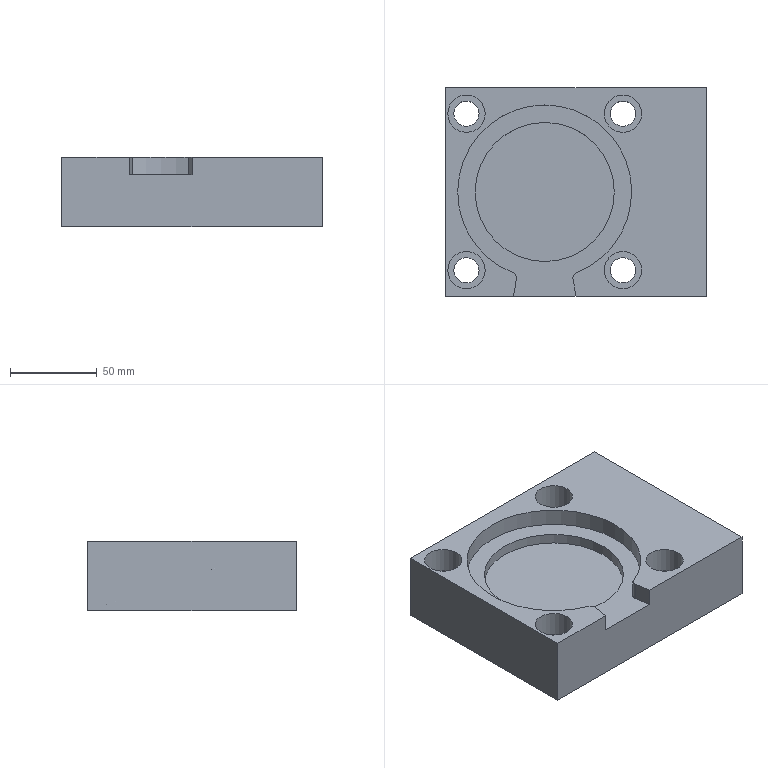NC program | NX | posted with a generic post | part box 150 x 120 x 40 mm
Lines 1855 to 1997 of 1997:
(ZLEVEL_PROFILE , TOOL : D6A45)
N3672 T07 M6
N3674 G54
N3676 G17 G0 G90 X28.082 Y52.851 S9500 M3
N3678 G43 Z30. H7
N3680 Z-0.667
N3682 G94 G1 Z-1.667 F1400.
N3684 X27.52 Y53.825
N3686 G3 X27. Y54.125 R0.6
N3688 X17.875 Y45. R9.125
N3690 X27. Y54.125 R-9.125
N3692 X26.48 Y53.825 R0.6
N3694 G1 X25.918 Y52.851
N3696 Z-0.667
N3698 G0 Z30.
N3700 X28.11 Y49.977
N3702 Z-15.
N3704 G1 Z-16.
N3706 X27.52 Y50.999
N3708 G3 X27. Y51.299 R0.6
N3710 X20.701 Y45. R6.299
N3712 X27. Y51.299 R-6.299
N3714 X26.48 Y50.999 R0.6
N3716 G1 X25.89 Y49.977
N3718 Z-15.
N3720 G0 Z30.
N3722 X-61.918 Y52.851
N3724 Z-0.667
N3726 G1 Z-1.667
N3728 X-62.48 Y53.825
N3730 G3 X-63. Y54.125 R0.6
N3732 X-72.125 Y45. R9.125
N3734 X-63. Y54.125 R-9.125
N3736 X-63.52 Y53.825 R0.6
N3738 G1 X-64.082 Y52.851
N3740 Z-0.667
N3742 G0 Z30.
N3744 X-61.89 Y49.977
N3746 Z-15.
N3748 G1 Z-16.
N3750 X-62.48 Y50.999
N3752 G3 X-63. Y51.299 R0.6
N3754 X-69.299 Y45. R6.299
N3756 X-63. Y51.299 R-6.299
N3758 X-63.52 Y50.999 R0.6
N3760 G1 X-64.11 Y49.977
N3762 Z-15.
N3764 G0 Z30.
N3766 X25.918 Y-52.851
N3768 Z-0.667
N3770 G1 Z-1.667
N3772 X26.48 Y-53.825
N3774 G3 X27. Y-54.125 R0.6
N3776 X36.125 Y-45. R9.125
N3778 X27. Y-54.125 R-9.125
N3780 X27.52 Y-53.825 R0.6
N3782 G1 X28.082 Y-52.851
N3784 Z-0.667
N3786 G0 Z30.
N3788 X25.89 Y-49.977
N3790 Z-15.
N3792 G1 Z-16.
N3794 X26.48 Y-50.999
N3796 G3 X27. Y-51.299 R0.6
N3798 X33.299 Y-45. R6.299
N3800 X27. Y-51.299 R-6.299
N3802 X27.52 Y-50.999 R0.6
N3804 G1 X28.11 Y-49.977
N3806 Z-15.
N3808 G0 Z30.
N3810 X-64.082 Y-52.851
N3812 Z-0.667
N3814 G1 Z-1.667
N3816 X-63.52 Y-53.825
N3818 G3 X-63. Y-54.125 R0.6
N3820 X-53.875 Y-45. R9.125
N3822 X-63. Y-54.125 R-9.125
N3824 X-62.48 Y-53.825 R0.6
N3826 G1 X-61.918 Y-52.851
N3828 Z-0.667
N3830 G0 Z30.
N3832 X-64.11 Y-49.977
N3834 Z-15.
N3836 G1 Z-16.
N3838 X-63.52 Y-50.999
N3840 G3 X-63. Y-51.299 R0.6
N3842 X-56.701 Y-45. R6.299
N3844 X-63. Y-51.299 R-6.299
N3846 X-62.48 Y-50.999 R0.6
N3848 G1 X-61.89 Y-49.977
N3850 Z-15.
N3852 G0 Z30.
N3854 X-1.039 Y62.825
N3856 Z-0.667
N3858 G1 Z-1.667
N3860 X-0.52 Y61.925
N3862 G3 X0. Y61.625 R0.6
N3864 G1 X75.002
N3866 G2 X76.625 Y60.003 R1.623
N3868 G1 Y-60.003
N3870 G2 X75.002 Y-61.625 R1.623
N3872 G1 X-0.015
N3874 G2 X-1.6 Y-60.285 R1.615
N3876 G1 X-3.376 Y-50.211
N3878 G2 X-0.495 Y-45.096 R4.625
N3880 G3 X-35.505 Y-45.096 R-48.375
N3882 G2 X-32.624 Y-50.211 R4.625
N3884 G1 X-34.4 Y-60.285
N3886 G2 X-35.997 Y-61.625 R1.622
N3888 G1 X-75.002
N3890 G2 X-76.625 Y-60.003 R1.623
N3892 G1 Y60.003
N3894 G2 X-75.002 Y61.625 R1.623
N3896 G1 X0.
N3898 G3 X0.52 Y61.925 R0.6
N3900 G1 X1.039 Y62.825
N3902 Z-0.667
N3904 G0 Z30.
N3906 X-1.744 Y-63.711
N3908 Z-10.667
N3910 G1 Z-11.667
N3912 X-2.861 Y-61.775
N3914 G3 X-3.121 Y-61.625 R0.3
N3916 G1 X-32.89
N3918 G3 X-33.15 Y-61.775 R0.3
N3920 G1 X-34.271 Y-63.718
N3922 Z-10.667
N3924 G0 Z30.
N3926 X-55.16 Y1.048
N3928 Z-10.667
N3930 G1 Z-11.667
N3932 X-56.075 Y0.52
N3934 G3 X-56.375 Y0. R0.6
N3936 X-18. Y-38.375 R38.375
N3938 X-56.375 Y0. R-38.375
N3940 X-56.075 Y-0.52 R0.6
N3942 G1 X-55.16 Y-1.048
N3944 Z-10.667
N3946 G0 Z30.
N3948 M5
N3950 M2